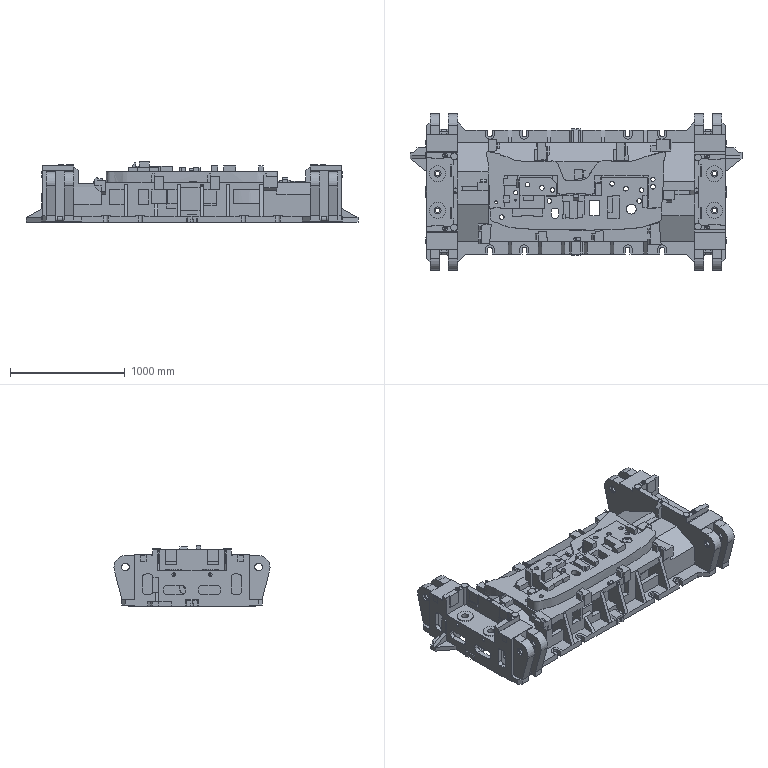Part | NX | features solid 2 | 1 solid | 1705 faces | box 2890 x 1360 x 525 mm | volume 422714533 mm3 | plane 1374 | cylinder 286 | spline 35 | torus 8 | cone 2 | commonest cylinder face diameters 60 x111 68 x48 40 x46 30 x18 64 x16 80 x8